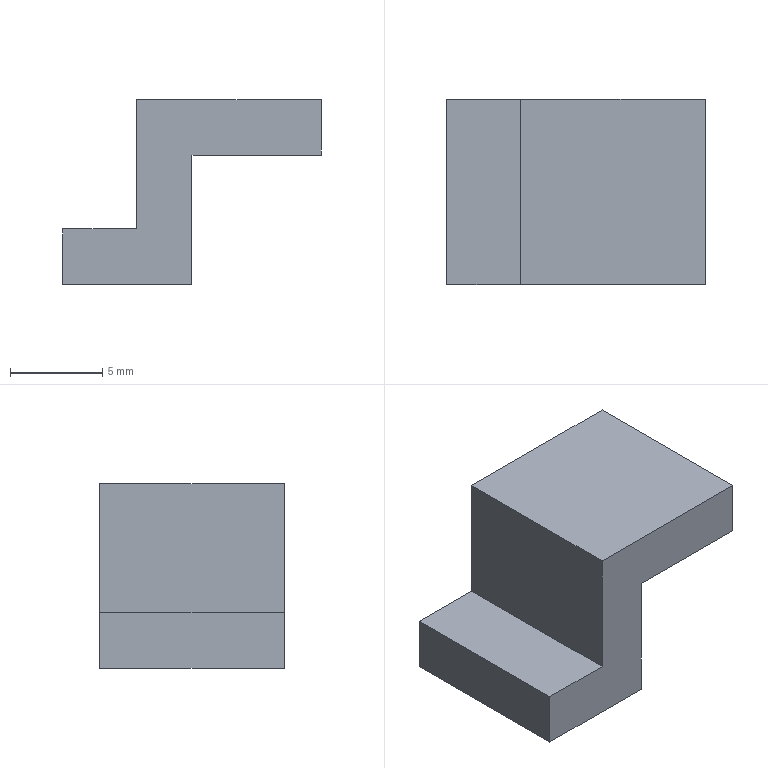Part | SolidWorks | features Extrusion 1 | 1 solid | 10 faces | box 14 x 10 x 10 mm | volume 630 mm3 | plane 10
STEP:
#1=CARTESIAN_POINT('',(0.,0.,-3.));
#2=VERTEX_POINT('',#1);
#3=CARTESIAN_POINT('',(0.,0.,0.));
#4=VERTEX_POINT('',#3);
#5=CARTESIAN_POINT('',(0.,0.,-3.));
#6=DIRECTION('',(0.,0.,1.));
#7=VECTOR('',#6,1000.);
#8=LINE('',#5,#7);
#9=EDGE_CURVE('',#2,#4,#8,.T.);
#10=ORIENTED_EDGE('',*,*,#9,.T.);
#11=CARTESIAN_POINT('',(0.,10.,0.));
#12=VERTEX_POINT('',#11);
#13=CARTESIAN_POINT('',(0.,10.,0.));
#14=DIRECTION('',(0.,-1.,0.));
#15=VECTOR('',#14,1000.);
#16=LINE('',#13,#15);
#17=EDGE_CURVE('',#12,#4,#16,.T.);
#18=ORIENTED_EDGE('',*,*,#17,.F.);
#19=CARTESIAN_POINT('',(0.,10.,-3.));
#20=VERTEX_POINT('',#19);
#21=CARTESIAN_POINT('',(0.,10.,-3.));
#22=DIRECTION('',(0.,0.,1.));
#23=VECTOR('',#22,1000.);
#24=LINE('',#21,#23);
#25=EDGE_CURVE('',#20,#12,#24,.T.);
#26=ORIENTED_EDGE('',*,*,#25,.F.);
#27=CARTESIAN_POINT('',(0.,10.,-3.));
#28=DIRECTION('',(0.,-1.,0.));
#29=VECTOR('',#28,1000.);
#30=LINE('',#27,#29);
#31=EDGE_CURVE('',#20,#2,#30,.T.);
#32=ORIENTED_EDGE('',*,*,#31,.T.);
#33=EDGE_LOOP('',(#10,#18,#26,#32));
#34=FACE_OUTER_BOUND('',#33,.T.);
#35=CARTESIAN_POINT('',(0.,10.,-3.));
#36=DIRECTION('',(1.,0.,0.));
#37=DIRECTION('',(0.,0.,-1.));
#38=AXIS2_PLACEMENT_3D('',#35,#36,#37);
#39=PLANE('',#38);
#40=ADVANCED_FACE('',(#34),#39,.F.);
#41=CARTESIAN_POINT('',(4.,0.,0.));
#42=VERTEX_POINT('',#41);
#43=CARTESIAN_POINT('',(0.,0.,0.));
#44=DIRECTION('',(1.,0.,0.));
#45=VECTOR('',#44,1000.);
#46=LINE('',#43,#45);
#47=EDGE_CURVE('',#4,#42,#46,.T.);
#48=ORIENTED_EDGE('',*,*,#47,.T.);
#49=CARTESIAN_POINT('',(4.,10.,0.));
#50=VERTEX_POINT('',#49);
#51=CARTESIAN_POINT('',(4.,10.,0.));
#52=DIRECTION('',(0.,-1.,0.));
#53=VECTOR('',#52,1000.);
#54=LINE('',#51,#53);
#55=EDGE_CURVE('',#50,#42,#54,.T.);
#56=ORIENTED_EDGE('',*,*,#55,.F.);
#57=CARTESIAN_POINT('',(0.,10.,0.));
#58=DIRECTION('',(1.,0.,0.));
#59=VECTOR('',#58,1000.);
#60=LINE('',#57,#59);
#61=EDGE_CURVE('',#12,#50,#60,.T.);
#62=ORIENTED_EDGE('',*,*,#61,.F.);
#63=ORIENTED_EDGE('',*,*,#17,.T.);
#64=EDGE_LOOP('',(#48,#56,#62,#63));
#65=FACE_OUTER_BOUND('',#64,.T.);
#66=CARTESIAN_POINT('',(0.,10.,0.));
#67=DIRECTION('',(0.,0.,-1.));
#68=DIRECTION('',(-1.,0.,0.));
#69=AXIS2_PLACEMENT_3D('',#66,#67,#68);
#70=PLANE('',#69);
#71=ADVANCED_FACE('',(#65),#70,.F.);
#72=CARTESIAN_POINT('',(4.,0.,7.));
#73=VERTEX_POINT('',#72);
#74=CARTESIAN_POINT('',(4.,0.,0.));
#75=DIRECTION('',(0.,0.,1.));
#76=VECTOR('',#75,1000.);
#77=LINE('',#74,#76);
#78=EDGE_CURVE('',#42,#73,#77,.T.);
#79=ORIENTED_EDGE('',*,*,#78,.T.);
#80=CARTESIAN_POINT('',(4.,10.,7.));
#81=VERTEX_POINT('',#80);
#82=CARTESIAN_POINT('',(4.,10.,7.));
#83=DIRECTION('',(0.,-1.,0.));
#84=VECTOR('',#83,1000.);
#85=LINE('',#82,#84);
#86=EDGE_CURVE('',#81,#73,#85,.T.);
#87=ORIENTED_EDGE('',*,*,#86,.F.);
#88=CARTESIAN_POINT('',(4.,10.,0.));
#89=DIRECTION('',(0.,0.,1.));
#90=VECTOR('',#89,1000.);
#91=LINE('',#88,#90);
#92=EDGE_CURVE('',#50,#81,#91,.T.);
#93=ORIENTED_EDGE('',*,*,#92,.F.);
#94=ORIENTED_EDGE('',*,*,#55,.T.);
#95=EDGE_LOOP('',(#79,#87,#93,#94));
#96=FACE_OUTER_BOUND('',#95,.T.);
#97=CARTESIAN_POINT('',(4.,10.,0.));
#98=DIRECTION('',(1.,0.,0.));
#99=DIRECTION('',(0.,0.,-1.));
#100=AXIS2_PLACEMENT_3D('',#97,#98,#99);
#101=PLANE('',#100);
#102=ADVANCED_FACE('',(#96),#101,.F.);
#103=CARTESIAN_POINT('',(14.,0.,7.));
#104=VERTEX_POINT('',#103);
#105=CARTESIAN_POINT('',(4.,0.,7.));
#106=DIRECTION('',(1.,0.,0.));
#107=VECTOR('',#106,1000.);
#108=LINE('',#105,#107);
#109=EDGE_CURVE('',#73,#104,#108,.T.);
#110=ORIENTED_EDGE('',*,*,#109,.T.);
#111=CARTESIAN_POINT('',(14.,10.,7.));
#112=VERTEX_POINT('',#111);
#113=CARTESIAN_POINT('',(14.,10.,7.));
#114=DIRECTION('',(0.,-1.,0.));
#115=VECTOR('',#114,1000.);
#116=LINE('',#113,#115);
#117=EDGE_CURVE('',#112,#104,#116,.T.);
#118=ORIENTED_EDGE('',*,*,#117,.F.);
#119=CARTESIAN_POINT('',(4.,10.,7.));
#120=DIRECTION('',(1.,0.,0.));
#121=VECTOR('',#120,1000.);
#122=LINE('',#119,#121);
#123=EDGE_CURVE('',#81,#112,#122,.T.);
#124=ORIENTED_EDGE('',*,*,#123,.F.);
#125=ORIENTED_EDGE('',*,*,#86,.T.);
#126=EDGE_LOOP('',(#110,#118,#124,#125));
#127=FACE_OUTER_BOUND('',#126,.T.);
#128=CARTESIAN_POINT('',(4.,10.,7.));
#129=DIRECTION('',(0.,0.,-1.));
#130=DIRECTION('',(-1.,0.,0.));
#131=AXIS2_PLACEMENT_3D('',#128,#129,#130);
#132=PLANE('',#131);
#133=ADVANCED_FACE('',(#127),#132,.F.);
#134=CARTESIAN_POINT('',(14.,0.,4.));
#135=VERTEX_POINT('',#134);
#136=CARTESIAN_POINT('',(14.,0.,4.));
#137=DIRECTION('',(0.,0.,-1.));
#138=VECTOR('',#137,1000.);
#139=LINE('',#136,#138);
#140=EDGE_CURVE('',#104,#135,#139,.T.);
#141=ORIENTED_EDGE('',*,*,#140,.T.);
#142=CARTESIAN_POINT('',(14.,10.,4.));
#143=VERTEX_POINT('',#142);
#144=CARTESIAN_POINT('',(14.,10.,4.));
#145=DIRECTION('',(0.,-1.,0.));
#146=VECTOR('',#145,1000.);
#147=LINE('',#144,#146);
#148=EDGE_CURVE('',#143,#135,#147,.T.);
#149=ORIENTED_EDGE('',*,*,#148,.F.);
#150=CARTESIAN_POINT('',(14.,10.,4.));
#151=DIRECTION('',(0.,0.,-1.));
#152=VECTOR('',#151,1000.);
#153=LINE('',#150,#152);
#154=EDGE_CURVE('',#112,#143,#153,.T.);
#155=ORIENTED_EDGE('',*,*,#154,.F.);
#156=ORIENTED_EDGE('',*,*,#117,.T.);
#157=EDGE_LOOP('',(#141,#149,#155,#156));
#158=FACE_OUTER_BOUND('',#157,.T.);
#159=CARTESIAN_POINT('',(14.,10.,4.));
#160=DIRECTION('',(-1.,0.,0.));
#161=DIRECTION('',(0.,0.,1.));
#162=AXIS2_PLACEMENT_3D('',#159,#160,#161);
#163=PLANE('',#162);
#164=ADVANCED_FACE('',(#158),#163,.F.);
#165=CARTESIAN_POINT('',(7.,0.,4.));
#166=VERTEX_POINT('',#165);
#167=CARTESIAN_POINT('',(7.,0.,4.));
#168=DIRECTION('',(-1.,0.,0.));
#169=VECTOR('',#168,1000.);
#170=LINE('',#167,#169);
#171=EDGE_CURVE('',#135,#166,#170,.T.);
#172=ORIENTED_EDGE('',*,*,#171,.T.);
#173=CARTESIAN_POINT('',(7.,10.,4.));
#174=VERTEX_POINT('',#173);
#175=CARTESIAN_POINT('',(7.,10.,4.));
#176=DIRECTION('',(0.,-1.,0.));
#177=VECTOR('',#176,1000.);
#178=LINE('',#175,#177);
#179=EDGE_CURVE('',#174,#166,#178,.T.);
#180=ORIENTED_EDGE('',*,*,#179,.F.);
#181=CARTESIAN_POINT('',(7.,10.,4.));
#182=DIRECTION('',(-1.,0.,0.));
#183=VECTOR('',#182,1000.);
#184=LINE('',#181,#183);
#185=EDGE_CURVE('',#143,#174,#184,.T.);
#186=ORIENTED_EDGE('',*,*,#185,.F.);
#187=ORIENTED_EDGE('',*,*,#148,.T.);
#188=EDGE_LOOP('',(#172,#180,#186,#187));
#189=FACE_OUTER_BOUND('',#188,.T.);
#190=CARTESIAN_POINT('',(7.,10.,4.));
#191=DIRECTION('',(0.,0.,1.));
#192=DIRECTION('',(1.,0.,0.));
#193=AXIS2_PLACEMENT_3D('',#190,#191,#192);
#194=PLANE('',#193);
#195=ADVANCED_FACE('',(#189),#194,.F.);
#196=CARTESIAN_POINT('',(7.,0.,-3.));
#197=VERTEX_POINT('',#196);
#198=CARTESIAN_POINT('',(7.,0.,-3.));
#199=DIRECTION('',(0.,0.,-1.));
#200=VECTOR('',#199,1000.);
#201=LINE('',#198,#200);
#202=EDGE_CURVE('',#166,#197,#201,.T.);
#203=ORIENTED_EDGE('',*,*,#202,.T.);
#204=CARTESIAN_POINT('',(7.,10.,-3.));
#205=VERTEX_POINT('',#204);
#206=CARTESIAN_POINT('',(7.,10.,-3.));
#207=DIRECTION('',(0.,-1.,0.));
#208=VECTOR('',#207,1000.);
#209=LINE('',#206,#208);
#210=EDGE_CURVE('',#205,#197,#209,.T.);
#211=ORIENTED_EDGE('',*,*,#210,.F.);
#212=CARTESIAN_POINT('',(7.,10.,-3.));
#213=DIRECTION('',(0.,0.,-1.));
#214=VECTOR('',#213,1000.);
#215=LINE('',#212,#214);
#216=EDGE_CURVE('',#174,#205,#215,.T.);
#217=ORIENTED_EDGE('',*,*,#216,.F.);
#218=ORIENTED_EDGE('',*,*,#179,.T.);
#219=EDGE_LOOP('',(#203,#211,#217,#218));
#220=FACE_OUTER_BOUND('',#219,.T.);
#221=CARTESIAN_POINT('',(7.,10.,-3.));
#222=DIRECTION('',(-1.,0.,0.));
#223=DIRECTION('',(0.,0.,1.));
#224=AXIS2_PLACEMENT_3D('',#221,#222,#223);
#225=PLANE('',#224);
#226=ADVANCED_FACE('',(#220),#225,.F.);
#227=CARTESIAN_POINT('',(0.,0.,-3.));
#228=DIRECTION('',(-1.,0.,0.));
#229=VECTOR('',#228,1000.);
#230=LINE('',#227,#229);
#231=EDGE_CURVE('',#197,#2,#230,.T.);
#232=ORIENTED_EDGE('',*,*,#231,.T.);
#233=ORIENTED_EDGE('',*,*,#31,.F.);
#234=CARTESIAN_POINT('',(0.,10.,-3.));
#235=DIRECTION('',(-1.,0.,0.));
#236=VECTOR('',#235,1000.);
#237=LINE('',#234,#236);
#238=EDGE_CURVE('',#205,#20,#237,.T.);
#239=ORIENTED_EDGE('',*,*,#238,.F.);
#240=ORIENTED_EDGE('',*,*,#210,.T.);
#241=EDGE_LOOP('',(#232,#233,#239,#240));
#242=FACE_OUTER_BOUND('',#241,.T.);
#243=CARTESIAN_POINT('',(0.,10.,-3.));
#244=DIRECTION('',(0.,0.,1.));
#245=DIRECTION('',(1.,0.,0.));
#246=AXIS2_PLACEMENT_3D('',#243,#244,#245);
#247=PLANE('',#246);
#248=ADVANCED_FACE('',(#242),#247,.F.);
#249=ORIENTED_EDGE('',*,*,#25,.T.);
#250=ORIENTED_EDGE('',*,*,#61,.T.);
#251=ORIENTED_EDGE('',*,*,#92,.T.);
#252=ORIENTED_EDGE('',*,*,#123,.T.);
#253=ORIENTED_EDGE('',*,*,#154,.T.);
#254=ORIENTED_EDGE('',*,*,#185,.T.);
#255=ORIENTED_EDGE('',*,*,#216,.T.);
#256=ORIENTED_EDGE('',*,*,#238,.T.);
#257=EDGE_LOOP('',(#249,#250,#251,#252,#253,#254,#255,#256));
#258=FACE_OUTER_BOUND('',#257,.T.);
#259=CARTESIAN_POINT('',(0.,10.,0.));
#260=DIRECTION('',(0.,1.,0.));
#261=DIRECTION('',(0.,0.,1.));
#262=AXIS2_PLACEMENT_3D('',#259,#260,#261);
#263=PLANE('',#262);
#264=ADVANCED_FACE('',(#258),#263,.T.);
#265=ORIENTED_EDGE('',*,*,#9,.F.);
#266=ORIENTED_EDGE('',*,*,#231,.F.);
#267=ORIENTED_EDGE('',*,*,#202,.F.);
#268=ORIENTED_EDGE('',*,*,#171,.F.);
#269=ORIENTED_EDGE('',*,*,#140,.F.);
#270=ORIENTED_EDGE('',*,*,#109,.F.);
#271=ORIENTED_EDGE('',*,*,#78,.F.);
#272=ORIENTED_EDGE('',*,*,#47,.F.);
#273=EDGE_LOOP('',(#265,#266,#267,#268,#269,#270,#271,#272));
#274=FACE_OUTER_BOUND('',#273,.T.);
#275=CARTESIAN_POINT('',(0.,0.,0.));
#276=DIRECTION('',(0.,1.,0.));
#277=DIRECTION('',(0.,0.,1.));
#278=AXIS2_PLACEMENT_3D('',#275,#276,#277);
#279=PLANE('',#278);
#280=ADVANCED_FACE('',(#274),#279,.F.);
#281=CLOSED_SHELL('',(#40,#71,#102,#133,#164,#195,#226,#248,#264,#280));
#282=MANIFOLD_SOLID_BREP('',#281);
#283=CARTESIAN_POINT('',(0.,0.,0.));
#284=DIRECTION('',(0.,0.,1.));
#285=DIRECTION('',(1.,0.,0.));
#286=AXIS2_PLACEMENT_3D('',#283,#284,#285);
#287=(LENGTH_UNIT()NAMED_UNIT(*)SI_UNIT(.MILLI.,.METRE.));
#288=UNCERTAINTY_MEASURE_WITH_UNIT(LENGTH_MEASURE(0.00001),#287,'','');
#289=(NAMED_UNIT(*)PLANE_ANGLE_UNIT()SI_UNIT($,.RADIAN.));
#290=(NAMED_UNIT(*)SI_UNIT($,.STERADIAN.)SOLID_ANGLE_UNIT());
#291=(GEOMETRIC_REPRESENTATION_CONTEXT(3)GLOBAL_UNCERTAINTY_ASSIGNED_CONTEXT((#288))GLOBAL_UNIT_ASSIGNED_CONTEXT((#287,#289,#290))REPRESENTATION_CONTEXT('',''));
#292=ADVANCED_BREP_SHAPE_REPRESENTATION('',(#282,#286),#291);